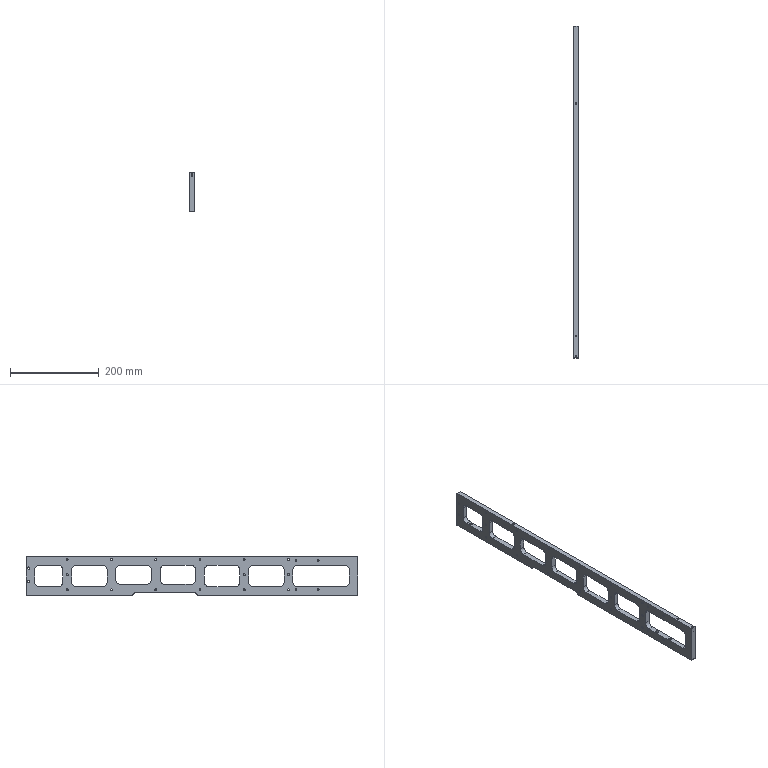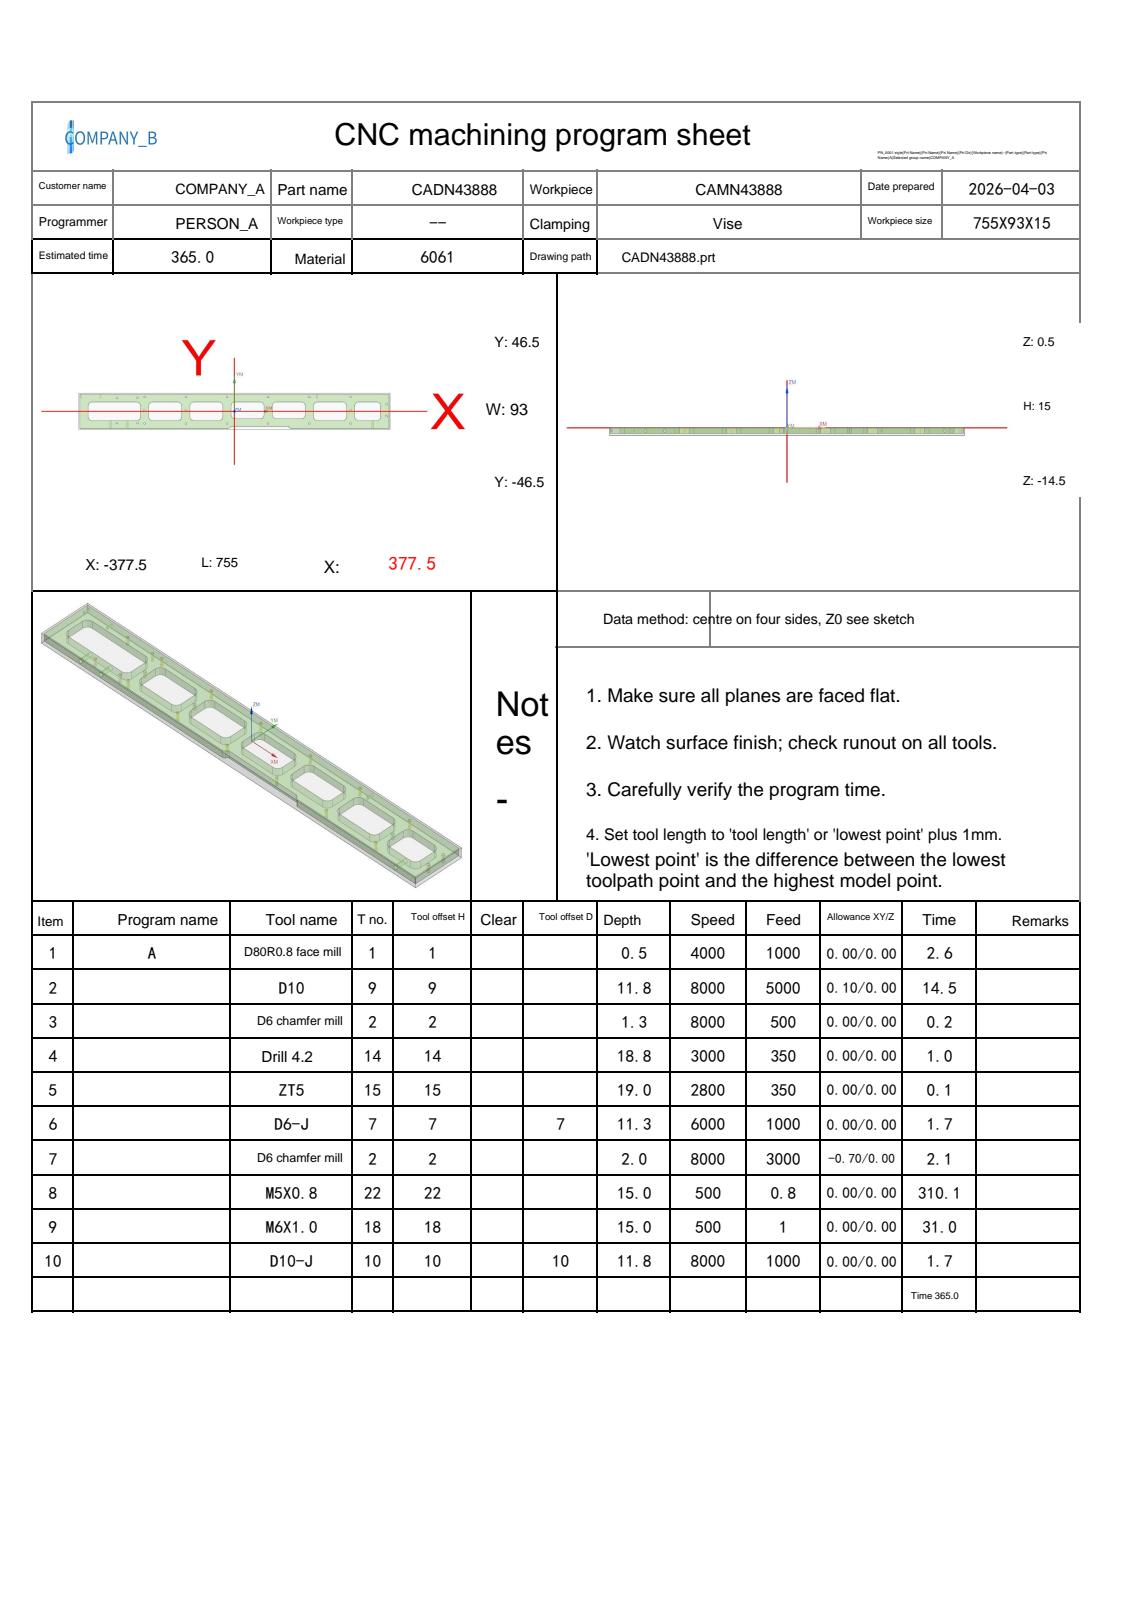NC program | NX | posted by the shop | part box 11 x 750 x 88 mm
Lines 1 to 1861 of 2351, first 1298 of 1859 lines:
%
O0001
(Machine time: 686.22 MIN)
(===Total Tool:9===)
(T1=D80R0.8 face mill D=80.  R=0.8  D-  H01 Z=-0.   )
(T9=D10     D=10.  R=0.   D-  H09 Z=-11.3 )
(T2=D6 chamfer mill   D=6.   R=0.   D-  H02 Z=-1.5  )
(T14=drill 4.2  D=4.2  DR_a=118 D-  H14 Z=-18.26)
(T15=ZT5    D=5.   DR_a=118 D-  H15 Z=-18.5 )
(T7=D6-J    D=6.   R=0.   D7  H07 Z=-10.8 )
(T22=M5X0.8 D=4.2  DR_a=180 D-  H22 Z=-14.5 )
(T18=M6X1.0 D=5.   DR_a=180 D-  H18 Z=-14.5 )
(T10=D10-J  D=10.  R=0.   D10 H10 Z=-11.3 )
G80 G90 G17 G49 G40
G91 G28 Z0
M01
N1 T01 M06
(D80R0.8 face mill  D=80. R=0.8 H=01 ce=0.00 di=0.00)
G00 G90 G54 X-420. Y42. M03 S4000
G43 H01 Z20.
M08
Z2.
G01 Z0.0 F1000.
X-415.
X415.
Y0.0
X-415.
Y-42.
X415.
X420.
Z2.
G00 Z20.
G91 G28 Z0.0
M05
M09
G91 G28 Z0.0
M01
N2 T09 M06
(D10  D=10. R=0. H=09 ce=0.10 di=0.00)
G00 G90 G54 X0.0 Y49.1 M03 S8000
G43 H09 Z20.
M08
Z.5
G01 X374. Z.328 F5000.
G02 X380.1 Y43. Z.324 I0.0 J-6.1
G01 Y-43. Z.284
G02 X374. Y-49.1 Z.28 I-6.1 J0.0
G01 X137.165 Z.171
G02 X127.935 Y-43.1 Z.165 I0.0 J10.1
G01 X-5.935 Z.104
G02 X-15.165 Y-49.1 Z.099 I-9.23 J4.1
G01 X-374. Z-.066
G02 X-380.1 Y-43. Z-.071 I0.0 J6.1
G01 Y43. Z-.11
G02 X-374. Y49.1 Z-.115 I6.1 J0.0
G01 X374. Z-.459
G02 X380.1 Y43. Z-.463 I0.0 J-6.1
G01 Y-43. Z-.503
G02 X374. Y-49.1 Z-.507 I-6.1 J0.0
G01 X137.165 Z-.616
G02 X127.935 Y-43.1 Z-.621 I0.0 J10.1
G01 X-5.935 Z-.683
G02 X-15.165 Y-49.1 Z-.688 I-9.23 J4.1
G01 X-374. Z-.853
G02 X-380.1 Y-43. Z-.857 I0.0 J6.1
G01 Y43. Z-.897
G02 X-374. Y49.1 Z-.901 I6.1 J0.0
G01 X374. Z-1.245
G02 X380.1 Y43. Z-1.25 I0.0 J-6.1
G01 Y-43. Z-1.289
G02 X374. Y-49.1 Z-1.294 I-6.1 J0.0
G01 X137.165 Z-1.402
G02 X127.935 Y-43.1 Z-1.408 I0.0 J10.1
G01 X-5.935 Z-1.469
G02 X-15.165 Y-49.1 Z-1.475 I-9.23 J4.1
G01 X-374. Z-1.64
G02 X-380.1 Y-43. Z-1.644 I0.0 J6.1
G01 Y43. Z-1.684
G02 X-374. Y49.1 Z-1.688 I6.1 J0.0
G01 X374. Z-2.032
G02 X380.1 Y43. Z-2.036 I0.0 J-6.1
G01 Y-43. Z-2.076
G02 X374. Y-49.1 Z-2.08 I-6.1 J0.0
G01 X137.165 Z-2.189
G02 X127.935 Y-43.1 Z-2.195 I0.0 J10.1
G01 X-5.935 Z-2.256
G02 X-15.165 Y-49.1 Z-2.261 I-9.23 J4.1
G01 X-374. Z-2.426
G02 X-380.1 Y-43. Z-2.431 I0.0 J6.1
G01 Y43. Z-2.47
G02 X-374. Y49.1 Z-2.475 I6.1 J0.0
G01 X374. Z-2.819
G02 X380.1 Y43. Z-2.823 I0.0 J-6.1
G01 Y-43. Z-2.863
G02 X374. Y-49.1 Z-2.867 I-6.1 J0.0
G01 X137.165 Z-2.976
G02 X127.935 Y-43.1 Z-2.981 I0.0 J10.1
G01 X-5.935 Z-3.043
G02 X-15.165 Y-49.1 Z-3.048 I-9.23 J4.1
G01 X-374. Z-3.213
G02 X-380.1 Y-43. Z-3.217 I0.0 J6.1
G01 Y43. Z-3.257
G02 X-374. Y49.1 Z-3.261 I6.1 J0.0
G01 X374. Z-3.605
G02 X380.1 Y43. Z-3.61 I0.0 J-6.1
G01 Y-43. Z-3.649
G02 X374. Y-49.1 Z-3.654 I-6.1 J0.0
G01 X137.165 Z-3.762
G02 X127.935 Y-43.1 Z-3.768 I0.0 J10.1
G01 X-5.935 Z-3.829
G02 X-15.165 Y-49.1 Z-3.835 I-9.23 J4.1
G01 X-374. Z-4.
G02 X-380.1 Y-43. Z-4.004 I0.0 J6.1
G01 Y43. Z-4.044
G02 X-374. Y49.1 Z-4.048 I6.1 J0.0
G01 X374. Z-4.392
G02 X380.1 Y43. Z-4.396 I0.0 J-6.1
G01 Y-43. Z-4.436
G02 X374. Y-49.1 Z-4.44 I-6.1 J0.0
G01 X137.165 Z-4.549
G02 X127.935 Y-43.1 Z-4.555 I0.0 J10.1
G01 X-5.935 Z-4.616
G02 X-15.165 Y-49.1 Z-4.621 I-9.23 J4.1
G01 X-374. Z-4.786
G02 X-380.1 Y-43. Z-4.791 I0.0 J6.1
G01 Y43. Z-4.83
G02 X-374. Y49.1 Z-4.835 I6.1 J0.0
G01 X374. Z-5.179
G02 X380.1 Y43. Z-5.183 I0.0 J-6.1
G01 Y-43. Z-5.223
G02 X374. Y-49.1 Z-5.227 I-6.1 J0.0
G01 X137.165 Z-5.336
G02 X127.935 Y-43.1 Z-5.341 I0.0 J10.1
G01 X-5.935 Z-5.403
G02 X-15.165 Y-49.1 Z-5.408 I-9.23 J4.1
G01 X-374. Z-5.573
G02 X-380.1 Y-43. Z-5.577 I0.0 J6.1
G01 Y43. Z-5.617
G02 X-374. Y49.1 Z-5.621 I6.1 J0.0
G01 X374. Z-5.965
G02 X380.1 Y43. Z-5.97 I0.0 J-6.1
G01 Y-43. Z-6.009
G02 X374. Y-49.1 Z-6.014 I-6.1 J0.0
G01 X137.165 Z-6.122
G02 X127.935 Y-43.1 Z-6.128 I0.0 J10.1
G01 X-5.935 Z-6.189
G02 X-15.165 Y-49.1 Z-6.195 I-9.23 J4.1
G01 X-374. Z-6.36
G02 X-380.1 Y-43. Z-6.364 I0.0 J6.1
G01 Y43. Z-6.404
G02 X-374. Y49.1 Z-6.408 I6.1 J0.0
G01 X374. Z-6.752
G02 X380.1 Y43. Z-6.756 I0.0 J-6.1
G01 Y-43. Z-6.796
G02 X374. Y-49.1 Z-6.8 I-6.1 J0.0
G01 X137.165 Z-6.909
G02 X127.935 Y-43.1 Z-6.915 I0.0 J10.1
G01 X-5.935 Z-6.976
G02 X-15.165 Y-49.1 Z-6.981 I-9.23 J4.1
G01 X-374. Z-7.146
G02 X-380.1 Y-43. Z-7.151 I0.0 J6.1
G01 Y43. Z-7.19
G02 X-374. Y49.1 Z-7.195 I6.1 J0.0
G01 X374. Z-7.539
G02 X380.1 Y43. Z-7.543 I0.0 J-6.1
G01 Y-43. Z-7.583
G02 X374. Y-49.1 Z-7.587 I-6.1 J0.0
G01 X137.165 Z-7.696
G02 X127.935 Y-43.1 Z-7.701 I0.0 J10.1
G01 X-5.935 Z-7.763
G02 X-15.165 Y-49.1 Z-7.768 I-9.23 J4.1
G01 X-374. Z-7.933
G02 X-380.1 Y-43. Z-7.937 I0.0 J6.1
G01 Y43. Z-7.977
G02 X-374. Y49.1 Z-7.981 I6.1 J0.0
G01 X374. Z-8.325
G02 X380.1 Y43. Z-8.33 I0.0 J-6.1
G01 Y-43. Z-8.369
G02 X374. Y-49.1 Z-8.374 I-6.1 J0.0
G01 X137.165 Z-8.482
G02 X127.935 Y-43.1 Z-8.488 I0.0 J10.1
G01 X-5.935 Z-8.549
G02 X-15.165 Y-49.1 Z-8.555 I-9.23 J4.1
G01 X-374. Z-8.72
G02 X-380.1 Y-43. Z-8.724 I0.0 J6.1
G01 Y43. Z-8.764
G02 X-374. Y49.1 Z-8.768 I6.1 J0.0
G01 X374. Z-9.112
G02 X380.1 Y43. Z-9.116 I0.0 J-6.1
G01 Y-43. Z-9.156
G02 X374. Y-49.1 Z-9.16 I-6.1 J0.0
G01 X137.165 Z-9.269
G02 X127.935 Y-43.1 Z-9.275 I0.0 J10.1
G01 X-5.935 Z-9.336
G02 X-15.165 Y-49.1 Z-9.341 I-9.23 J4.1
G01 X-374. Z-9.506
G02 X-380.1 Y-43. Z-9.511 I0.0 J6.1
G01 Y43. Z-9.55
G02 X-374. Y49.1 Z-9.555 I6.1 J0.0
G01 X374. Z-9.899
G02 X380.1 Y43. Z-9.903 I0.0 J-6.1
G01 Y-43. Z-9.943
G02 X374. Y-49.1 Z-9.947 I-6.1 J0.0
G01 X137.165 Z-10.056
G02 X127.935 Y-43.1 Z-10.061 I0.0 J10.1
G01 X-5.935 Z-10.123
G02 X-15.165 Y-49.1 Z-10.128 I-9.23 J4.1
G01 X-374. Z-10.293
G02 X-380.1 Y-43. Z-10.297 I0.0 J6.1
G01 Y43. Z-10.337
G02 X-374. Y49.1 Z-10.341 I6.1 J0.0
G01 X374. Z-10.685
G02 X380.1 Y43. Z-10.69 I0.0 J-6.1
G01 Y-43. Z-10.729
G02 X374. Y-49.1 Z-10.734 I-6.1 J0.0
G01 X137.165 Z-10.842
G02 X127.935 Y-43.1 Z-10.848 I0.0 J10.1
G01 X-5.935 Z-10.909
G02 X-15.165 Y-49.1 Z-10.915 I-9.23 J4.1
G01 X-374. Z-11.08
G02 X-380.1 Y-43. Z-11.084 I0.0 J6.1
G01 Y43. Z-11.124
G02 X-374. Y49.1 Z-11.128 I6.1 J0.0
G01 X0.0 Z-11.3
X374.
G02 X380.1 Y43. I0.0 J-6.1
G01 Y-43.
G02 X374. Y-49.1 I-6.1 J0.0
G01 X137.165
G02 X127.935 Y-43.1 I0.0 J10.1
G01 X-5.935
G02 X-15.165 Y-49.1 I-9.23 J4.1
G01 X-374.
G02 X-380.1 Y-43. I0.0 J6.1
G01 Y43.
G02 X-374. Y49.1 I6.1 J0.0
G01 X0.0
X.5
Z-10.3
G00 Z20.
G00 G90 X-291.5 Y-18.9 M03 S6000
Z20.
Z.5
G01 X-238. Z.413 F4000.
G03 X-233.1 Y-14. Z.4 I0.0 J4.9
G01 Y14. Z.354
G03 X-238. Y18.9 Z.342 I-4.9 J0.0
G01 X-345. Z.167
G03 X-349.9 Y14. Z.154 I0.0 J-4.9
G01 Y-14. Z.109
G03 X-345. Y-18.9 Z.096 I4.9 J0.0
G01 X-238. Z-.079
G03 X-233.1 Y-14. Z-.091 I0.0 J4.9
G01 Y14. Z-.137
G03 X-238. Y18.9 Z-.15 I-4.9 J0.0
G01 X-345. Z-.324
G03 X-349.9 Y14. Z-.337 I0.0 J-4.9
G01 Y-14. Z-.383
G03 X-345. Y-18.9 Z-.395 I4.9 J0.0
G01 X-238. Z-.57
G03 X-233.1 Y-14. Z-.583 I0.0 J4.9
G01 Y14. Z-.628
G03 X-238. Y18.9 Z-.641 I-4.9 J0.0
G01 X-345. Z-.816
G03 X-349.9 Y14. Z-.828 I0.0 J-4.9
G01 Y-14. Z-.874
G03 X-345. Y-18.9 Z-.887 I4.9 J0.0
G01 X-238. Z-1.061
G03 X-233.1 Y-14. Z-1.074 I0.0 J4.9
G01 Y14. Z-1.12
G03 X-238. Y18.9 Z-1.132 I-4.9 J0.0
G01 X-345. Z-1.307
G03 X-349.9 Y14. Z-1.32 I0.0 J-4.9
G01 Y-14. Z-1.365
G03 X-345. Y-18.9 Z-1.378 I4.9 J0.0
G01 X-238. Z-1.553
G03 X-233.1 Y-14. Z-1.565 I0.0 J4.9
G01 Y14. Z-1.611
G03 X-238. Y18.9 Z-1.623 I-4.9 J0.0
G01 X-345. Z-1.798
G03 X-349.9 Y14. Z-1.811 I0.0 J-4.9
G01 Y-14. Z-1.857
G03 X-345. Y-18.9 Z-1.869 I4.9 J0.0
G01 X-238. Z-2.044
G03 X-233.1 Y-14. Z-2.056 I0.0 J4.9
G01 Y14. Z-2.102
G03 X-238. Y18.9 Z-2.115 I-4.9 J0.0
G01 X-345. Z-2.29
G03 X-349.9 Y14. Z-2.302 I0.0 J-4.9
G01 Y-14. Z-2.348
G03 X-345. Y-18.9 Z-2.36 I4.9 J0.0
G01 X-238. Z-2.535
G03 X-233.1 Y-14. Z-2.548 I0.0 J4.9
G01 Y14. Z-2.594
G03 X-238. Y18.9 Z-2.606 I-4.9 J0.0
G01 X-345. Z-2.781
G03 X-349.9 Y14. Z-2.793 I0.0 J-4.9
G01 Y-14. Z-2.839
G03 X-345. Y-18.9 Z-2.852 I4.9 J0.0
G01 X-238. Z-3.027
G03 X-233.1 Y-14. Z-3.039 I0.0 J4.9
G01 Y14. Z-3.085
G03 X-238. Y18.9 Z-3.097 I-4.9 J0.0
G01 X-345. Z-3.272
G03 X-349.9 Y14. Z-3.285 I0.0 J-4.9
G01 Y-14. Z-3.33
G03 X-345. Y-18.9 Z-3.343 I4.9 J0.0
G01 X-238. Z-3.518
G03 X-233.1 Y-14. Z-3.53 I0.0 J4.9
G01 Y14. Z-3.576
G03 X-238. Y18.9 Z-3.589 I-4.9 J0.0
G01 X-345. Z-3.763
G03 X-349.9 Y14. Z-3.776 I0.0 J-4.9
G01 Y-14. Z-3.822
G03 X-345. Y-18.9 Z-3.834 I4.9 J0.0
G01 X-238. Z-4.009
G03 X-233.1 Y-14. Z-4.022 I0.0 J4.9
G01 Y14. Z-4.067
G03 X-238. Y18.9 Z-4.08 I-4.9 J0.0
G01 X-345. Z-4.255
G03 X-349.9 Y14. Z-4.267 I0.0 J-4.9
G01 Y-14. Z-4.313
G03 X-345. Y-18.9 Z-4.326 I4.9 J0.0
G01 X-238. Z-4.5
G03 X-233.1 Y-14. Z-4.513 I0.0 J4.9
G01 Y14. Z-4.559
G03 X-238. Y18.9 Z-4.571 I-4.9 J0.0
G01 X-345. Z-4.746
G03 X-349.9 Y14. Z-4.759 I0.0 J-4.9
G01 Y-14. Z-4.804
G03 X-345. Y-18.9 Z-4.817 I4.9 J0.0
G01 X-238. Z-4.992
G03 X-233.1 Y-14. Z-5.004 I0.0 J4.9
G01 Y14. Z-5.05
G03 X-238. Y18.9 Z-5.063 I-4.9 J0.0
G01 X-345. Z-5.237
G03 X-349.9 Y14. Z-5.25 I0.0 J-4.9
G01 Y-14. Z-5.296
G03 X-345. Y-18.9 Z-5.308 I4.9 J0.0
G01 X-238. Z-5.483
G03 X-233.1 Y-14. Z-5.496 I0.0 J4.9
G01 Y14. Z-5.541
G03 X-238. Y18.9 Z-5.554 I-4.9 J0.0
G01 X-345. Z-5.729
G03 X-349.9 Y14. Z-5.741 I0.0 J-4.9
G01 Y-14. Z-5.787
G03 X-345. Y-18.9 Z-5.8 I4.9 J0.0
G01 X-238. Z-5.974
G03 X-233.1 Y-14. Z-5.987 I0.0 J4.9
G01 Y14. Z-6.033
G03 X-238. Y18.9 Z-6.045 I-4.9 J0.0
G01 X-345. Z-6.22
G03 X-349.9 Y14. Z-6.233 I0.0 J-4.9
G01 Y-14. Z-6.278
G03 X-345. Y-18.9 Z-6.291 I4.9 J0.0
G01 X-238. Z-6.466
G03 X-233.1 Y-14. Z-6.478 I0.0 J4.9
G01 Y14. Z-6.524
G03 X-238. Y18.9 Z-6.537 I-4.9 J0.0
G01 X-345. Z-6.711
G03 X-349.9 Y14. Z-6.724 I0.0 J-4.9
G01 Y-14. Z-6.77
G03 X-345. Y-18.9 Z-6.782 I4.9 J0.0
G01 X-238. Z-6.957
G03 X-233.1 Y-14. Z-6.97 I0.0 J4.9
G01 Y14. Z-7.015
G03 X-238. Y18.9 Z-7.028 I-4.9 J0.0
G01 X-345. Z-7.203
G03 X-349.9 Y14. Z-7.215 I0.0 J-4.9
G01 Y-14. Z-7.261
G03 X-345. Y-18.9 Z-7.273 I4.9 J0.0
G01 X-238. Z-7.448
G03 X-233.1 Y-14. Z-7.461 I0.0 J4.9
G01 Y14. Z-7.507
G03 X-238. Y18.9 Z-7.519 I-4.9 J0.0
G01 X-345. Z-7.694
G03 X-349.9 Y14. Z-7.706 I0.0 J-4.9
G01 Y-14. Z-7.752
G03 X-345. Y-18.9 Z-7.765 I4.9 J0.0
G01 X-238. Z-7.94
G03 X-233.1 Y-14. Z-7.952 I0.0 J4.9
G01 Y14. Z-7.998
G03 X-238. Y18.9 Z-8.01 I-4.9 J0.0
G01 X-345. Z-8.185
G03 X-349.9 Y14. Z-8.198 I0.0 J-4.9
G01 Y-14. Z-8.244
G03 X-345. Y-18.9 Z-8.256 I4.9 J0.0
G01 X-238. Z-8.431
G03 X-233.1 Y-14. Z-8.443 I0.0 J4.9
G01 Y14. Z-8.489
G03 X-238. Y18.9 Z-8.502 I-4.9 J0.0
G01 X-345. Z-8.677
G03 X-349.9 Y14. Z-8.689 I0.0 J-4.9
G01 Y-14. Z-8.735
G03 X-345. Y-18.9 Z-8.747 I4.9 J0.0
G01 X-238. Z-8.922
G03 X-233.1 Y-14. Z-8.935 I0.0 J4.9
G01 Y14. Z-8.98
G03 X-238. Y18.9 Z-8.993 I-4.9 J0.0
G01 X-345. Z-9.168
G03 X-349.9 Y14. Z-9.18 I0.0 J-4.9
G01 Y-14. Z-9.226
G03 X-345. Y-18.9 Z-9.239 I4.9 J0.0
G01 X-238. Z-9.413
G03 X-233.1 Y-14. Z-9.426 I0.0 J4.9
G01 Y14. Z-9.472
G03 X-238. Y18.9 Z-9.484 I-4.9 J0.0
G01 X-345. Z-9.659
G03 X-349.9 Y14. Z-9.672 I0.0 J-4.9
G01 Y-14. Z-9.717
G03 X-345. Y-18.9 Z-9.73 I4.9 J0.0
G01 X-238. Z-9.905
G03 X-233.1 Y-14. Z-9.917 I0.0 J4.9
G01 Y14. Z-9.963
G03 X-238. Y18.9 Z-9.976 I-4.9 J0.0
G01 X-345. Z-10.15
G03 X-349.9 Y14. Z-10.163 I0.0 J-4.9
G01 Y-14. Z-10.209
G03 X-345. Y-18.9 Z-10.221 I4.9 J0.0
G01 X-238. Z-10.396
G03 X-233.1 Y-14. Z-10.409 I0.0 J4.9
G01 Y14. Z-10.454
G03 X-238. Y18.9 Z-10.467 I-4.9 J0.0
G01 X-345. Z-10.642
G03 X-349.9 Y14. Z-10.654 I0.0 J-4.9
G01 Y-14. Z-10.7
G03 X-345. Y-18.9 Z-10.713 I4.9 J0.0
G01 X-291.5 Z-10.8
X-238.
G03 X-233.1 Y-14. I0.0 J4.9
G01 Y14.
G03 X-238. Y18.9 I-4.9 J0.0
G01 X-345.
G03 X-349.9 Y14. I0.0 J-4.9
G01 Y-14.
G03 X-345. Y-18.9 I4.9 J0.0
G01 X-291.5
X-291.
Z-9.8
G00 Z20.
G00 G90 X-168. Y18.9 M03 S6000
Z20.
Z.5
G01 X-198. Z.429 F4000.
G03 X-202.9 Y14. Z.41 I0.0 J-4.9
G01 Y-14. Z.344
G03 X-198. Y-18.9 Z.326 I4.9 J0.0
G01 X-138. Z.183
G03 X-133.1 Y-14. Z.165 I0.0 J4.9
G01 Y14. Z.098
G03 X-138. Y18.9 Z.08 I-4.9 J0.0
G01 X-198. Z-.063
G03 X-202.9 Y14. Z-.081 I0.0 J-4.9
G01 Y-14. Z-.147
G03 X-198. Y-18.9 Z-.166 I4.9 J0.0
G01 X-138. Z-.308
G03 X-133.1 Y-14. Z-.327 I0.0 J4.9
G01 Y14. Z-.393
G03 X-138. Y18.9 Z-.411 I-4.9 J0.0
G01 X-198. Z-.554
G03 X-202.9 Y14. Z-.572 I0.0 J-4.9
G01 Y-14. Z-.639
G03 X-198. Y-18.9 Z-.657 I4.9 J0.0
G01 X-138. Z-.8
G03 X-133.1 Y-14. Z-.818 I0.0 J4.9
G01 Y14. Z-.884
G03 X-138. Y18.9 Z-.903 I-4.9 J0.0
G01 X-198. Z-1.045
G03 X-202.9 Y14. Z-1.063 I0.0 J-4.9
G01 Y-14. Z-1.13
G03 X-198. Y-18.9 Z-1.148 I4.9 J0.0
G01 X-138. Z-1.291
G03 X-133.1 Y-14. Z-1.309 I0.0 J4.9
G01 Y14. Z-1.376
G03 X-138. Y18.9 Z-1.394 I-4.9 J0.0
G01 X-198. Z-1.536
G03 X-202.9 Y14. Z-1.555 I0.0 J-4.9
G01 Y-14. Z-1.621
G03 X-198. Y-18.9 Z-1.64 I4.9 J0.0
G01 X-138. Z-1.782
G03 X-133.1 Y-14. Z-1.8 I0.0 J4.9
G01 Y14. Z-1.867
G03 X-138. Y18.9 Z-1.885 I-4.9 J0.0
G01 X-198. Z-2.028
G03 X-202.9 Y14. Z-2.046 I0.0 J-4.9
G01 Y-14. Z-2.113
G03 X-198. Y-18.9 Z-2.131 I4.9 J0.0
G01 X-138. Z-2.273
G03 X-133.1 Y-14. Z-2.292 I0.0 J4.9
G01 Y14. Z-2.358
G03 X-138. Y18.9 Z-2.377 I-4.9 J0.0
G01 X-198. Z-2.519
G03 X-202.9 Y14. Z-2.537 I0.0 J-4.9
G01 Y-14. Z-2.604
G03 X-198. Y-18.9 Z-2.622 I4.9 J0.0
G01 X-138. Z-2.765
G03 X-133.1 Y-14. Z-2.783 I0.0 J4.9
G01 Y14. Z-2.85
G03 X-138. Y18.9 Z-2.868 I-4.9 J0.0
G01 X-198. Z-3.01
G03 X-202.9 Y14. Z-3.029 I0.0 J-4.9
G01 Y-14. Z-3.095
G03 X-198. Y-18.9 Z-3.114 I4.9 J0.0
G01 X-138. Z-3.256
G03 X-133.1 Y-14. Z-3.274 I0.0 J4.9
G01 Y14. Z-3.341
G03 X-138. Y18.9 Z-3.359 I-4.9 J0.0
G01 X-198. Z-3.502
G03 X-202.9 Y14. Z-3.52 I0.0 J-4.9
G01 Y-14. Z-3.587
G03 X-198. Y-18.9 Z-3.605 I4.9 J0.0
G01 X-138. Z-3.747
G03 X-133.1 Y-14. Z-3.766 I0.0 J4.9
G01 Y14. Z-3.832
G03 X-138. Y18.9 Z-3.85 I-4.9 J0.0
G01 X-198. Z-3.993
G03 X-202.9 Y14. Z-4.011 I0.0 J-4.9
G01 Y-14. Z-4.078
G03 X-198. Y-18.9 Z-4.096 I4.9 J0.0
G01 X-138. Z-4.239
G03 X-133.1 Y-14. Z-4.257 I0.0 J4.9
G01 Y14. Z-4.323
G03 X-138. Y18.9 Z-4.342 I-4.9 J0.0
G01 X-198. Z-4.484
G03 X-202.9 Y14. Z-4.503 I0.0 J-4.9
G01 Y-14. Z-4.569
G03 X-198. Y-18.9 Z-4.587 I4.9 J0.0
G01 X-138. Z-4.73
G03 X-133.1 Y-14. Z-4.748 I0.0 J4.9
G01 Y14. Z-4.815
G03 X-138. Y18.9 Z-4.833 I-4.9 J0.0
G01 X-198. Z-4.976
G03 X-202.9 Y14. Z-4.994 I0.0 J-4.9
G01 Y-14. Z-5.06
G03 X-198. Y-18.9 Z-5.079 I4.9 J0.0
G01 X-138. Z-5.221
G03 X-133.1 Y-14. Z-5.24 I0.0 J4.9
G01 Y14. Z-5.306
G03 X-138. Y18.9 Z-5.324 I-4.9 J0.0
G01 X-198. Z-5.467
G03 X-202.9 Y14. Z-5.485 I0.0 J-4.9
G01 Y-14. Z-5.552
G03 X-198. Y-18.9 Z-5.57 I4.9 J0.0
G01 X-138. Z-5.713
G03 X-133.1 Y-14. Z-5.731 I0.0 J4.9
G01 Y14. Z-5.797
G03 X-138. Y18.9 Z-5.816 I-4.9 J0.0
G01 X-198. Z-5.958
G03 X-202.9 Y14. Z-5.977 I0.0 J-4.9
G01 Y-14. Z-6.043
G03 X-198. Y-18.9 Z-6.061 I4.9 J0.0
G01 X-138. Z-6.204
G03 X-133.1 Y-14. Z-6.222 I0.0 J4.9
G01 Y14. Z-6.289
G03 X-138. Y18.9 Z-6.307 I-4.9 J0.0
G01 X-198. Z-6.45
G03 X-202.9 Y14. Z-6.468 I0.0 J-4.9
G01 Y-14. Z-6.534
G03 X-198. Y-18.9 Z-6.553 I4.9 J0.0
G01 X-138. Z-6.695
G03 X-133.1 Y-14. Z-6.713 I0.0 J4.9
G01 Y14. Z-6.78
G03 X-138. Y18.9 Z-6.798 I-4.9 J0.0
G01 X-198. Z-6.941
G03 X-202.9 Y14. Z-6.959 I0.0 J-4.9
G01 Y-14. Z-7.026
G03 X-198. Y-18.9 Z-7.044 I4.9 J0.0
G01 X-138. Z-7.186
G03 X-133.1 Y-14. Z-7.205 I0.0 J4.9
G01 Y14. Z-7.271
G03 X-138. Y18.9 Z-7.29 I-4.9 J0.0
G01 X-198. Z-7.432
G03 X-202.9 Y14. Z-7.45 I0.0 J-4.9
G01 Y-14. Z-7.517
G03 X-198. Y-18.9 Z-7.535 I4.9 J0.0
G01 X-138. Z-7.678
G03 X-133.1 Y-14. Z-7.696 I0.0 J4.9
G01 Y14. Z-7.763
G03 X-138. Y18.9 Z-7.781 I-4.9 J0.0
G01 X-198. Z-7.923
G03 X-202.9 Y14. Z-7.942 I0.0 J-4.9
G01 Y-14. Z-8.008
G03 X-198. Y-18.9 Z-8.027 I4.9 J0.0
G01 X-138. Z-8.169
G03 X-133.1 Y-14. Z-8.187 I0.0 J4.9
G01 Y14. Z-8.254
G03 X-138. Y18.9 Z-8.272 I-4.9 J0.0
G01 X-198. Z-8.415
G03 X-202.9 Y14. Z-8.433 I0.0 J-4.9
G01 Y-14. Z-8.5
G03 X-198. Y-18.9 Z-8.518 I4.9 J0.0
G01 X-138. Z-8.66
G03 X-133.1 Y-14. Z-8.679 I0.0 J4.9
G01 Y14. Z-8.745
G03 X-138. Y18.9 Z-8.764 I-4.9 J0.0
G01 X-198. Z-8.906
G03 X-202.9 Y14. Z-8.924 I0.0 J-4.9
G01 Y-14. Z-8.991
G03 X-198. Y-18.9 Z-9.009 I4.9 J0.0
G01 X-138. Z-9.152
G03 X-133.1 Y-14. Z-9.17 I0.0 J4.9
G01 Y14. Z-9.237
G03 X-138. Y18.9 Z-9.255 I-4.9 J0.0
G01 X-198. Z-9.397
G03 X-202.9 Y14. Z-9.416 I0.0 J-4.9
G01 Y-14. Z-9.482
G03 X-198. Y-18.9 Z-9.5 I4.9 J0.0
G01 X-138. Z-9.643
G03 X-133.1 Y-14. Z-9.661 I0.0 J4.9
G01 Y14. Z-9.728
G03 X-138. Y18.9 Z-9.746 I-4.9 J0.0
G01 X-198. Z-9.889
G03 X-202.9 Y14. Z-9.907 I0.0 J-4.9
G01 Y-14. Z-9.973
G03 X-198. Y-18.9 Z-9.992 I4.9 J0.0
G01 X-138. Z-10.134
G03 X-133.1 Y-14. Z-10.153 I0.0 J4.9
G01 Y14. Z-10.219
G03 X-138. Y18.9 Z-10.237 I-4.9 J0.0
G01 X-198. Z-10.38
G03 X-202.9 Y14. Z-10.398 I0.0 J-4.9
G01 Y-14. Z-10.465
G03 X-198. Y-18.9 Z-10.483 I4.9 J0.0
G01 X-138. Z-10.626
G03 X-133.1 Y-14. Z-10.644 I0.0 J4.9
G01 Y14. Z-10.71
G03 X-138. Y18.9 Z-10.729 I-4.9 J0.0
G01 X-168. Z-10.8
X-198.
G03 X-202.9 Y14. I0.0 J-4.9
G01 Y-14.
G03 X-198. Y-18.9 I4.9 J0.0
G01 X-138.
G03 X-133.1 Y-14. I0.0 J4.9
G01 Y14.
G03 X-138. Y18.9 I-4.9 J0.0
G01 X-168.
X-168.5
Z-9.8
G00 Z20.
X-68.
Z.5
G01 X-98. Z.429
G03 X-102.9 Y14. Z.41 I0.0 J-4.9
G01 Y-14. Z.344
G03 X-98. Y-18.9 Z.326 I4.9 J0.0
G01 X-38. Z.183
G03 X-33.1 Y-14. Z.165 I0.0 J4.9
G01 Y14. Z.098
G03 X-38. Y18.9 Z.08 I-4.9 J0.0
G01 X-98. Z-.063
G03 X-102.9 Y14. Z-.081 I0.0 J-4.9
G01 Y-14. Z-.147
G03 X-98. Y-18.9 Z-.166 I4.9 J0.0
G01 X-38. Z-.308
G03 X-33.1 Y-14. Z-.327 I0.0 J4.9
G01 Y14. Z-.393
G03 X-38. Y18.9 Z-.411 I-4.9 J0.0
G01 X-98. Z-.554
G03 X-102.9 Y14. Z-.572 I0.0 J-4.9
G01 Y-14. Z-.639
G03 X-98. Y-18.9 Z-.657 I4.9 J0.0
G01 X-38. Z-.8
G03 X-33.1 Y-14. Z-.818 I0.0 J4.9
G01 Y14. Z-.884
G03 X-38. Y18.9 Z-.903 I-4.9 J0.0
G01 X-98. Z-1.045
G03 X-102.9 Y14. Z-1.063 I0.0 J-4.9
G01 Y-14. Z-1.13
G03 X-98. Y-18.9 Z-1.148 I4.9 J0.0
G01 X-38. Z-1.291
G03 X-33.1 Y-14. Z-1.309 I0.0 J4.9
G01 Y14. Z-1.376
G03 X-38. Y18.9 Z-1.394 I-4.9 J0.0
G01 X-98. Z-1.536
G03 X-102.9 Y14. Z-1.555 I0.0 J-4.9
G01 Y-14. Z-1.621
G03 X-98. Y-18.9 Z-1.64 I4.9 J0.0
G01 X-38. Z-1.782
G03 X-33.1 Y-14. Z-1.8 I0.0 J4.9
G01 Y14. Z-1.867
G03 X-38. Y18.9 Z-1.885 I-4.9 J0.0
G01 X-98. Z-2.028
G03 X-102.9 Y14. Z-2.046 I0.0 J-4.9
G01 Y-14. Z-2.113
G03 X-98. Y-18.9 Z-2.131 I4.9 J0.0
G01 X-38. Z-2.273
G03 X-33.1 Y-14. Z-2.292 I0.0 J4.9
G01 Y14. Z-2.358
G03 X-38. Y18.9 Z-2.377 I-4.9 J0.0
G01 X-98. Z-2.519
G03 X-102.9 Y14. Z-2.537 I0.0 J-4.9
G01 Y-14. Z-2.604
G03 X-98. Y-18.9 Z-2.622 I4.9 J0.0
G01 X-38. Z-2.765
G03 X-33.1 Y-14. Z-2.783 I0.0 J4.9
G01 Y14. Z-2.85
G03 X-38. Y18.9 Z-2.868 I-4.9 J0.0
G01 X-98. Z-3.01
G03 X-102.9 Y14. Z-3.029 I0.0 J-4.9
G01 Y-14. Z-3.095
G03 X-98. Y-18.9 Z-3.114 I4.9 J0.0
G01 X-38. Z-3.256
G03 X-33.1 Y-14. Z-3.274 I0.0 J4.9
G01 Y14. Z-3.341
G03 X-38. Y18.9 Z-3.359 I-4.9 J0.0
G01 X-98. Z-3.502
G03 X-102.9 Y14. Z-3.52 I0.0 J-4.9
G01 Y-14. Z-3.587
G03 X-98. Y-18.9 Z-3.605 I4.9 J0.0
G01 X-38. Z-3.747
G03 X-33.1 Y-14. Z-3.766 I0.0 J4.9
G01 Y14. Z-3.832
G03 X-38. Y18.9 Z-3.85 I-4.9 J0.0
G01 X-98. Z-3.993
G03 X-102.9 Y14. Z-4.011 I0.0 J-4.9
G01 Y-14. Z-4.078
G03 X-98. Y-18.9 Z-4.096 I4.9 J0.0
G01 X-38. Z-4.239
G03 X-33.1 Y-14. Z-4.257 I0.0 J4.9
G01 Y14. Z-4.323
G03 X-38. Y18.9 Z-4.342 I-4.9 J0.0
G01 X-98. Z-4.484
G03 X-102.9 Y14. Z-4.503 I0.0 J-4.9
G01 Y-14. Z-4.569
G03 X-98. Y-18.9 Z-4.587 I4.9 J0.0
G01 X-38. Z-4.73
G03 X-33.1 Y-14. Z-4.748 I0.0 J4.9
G01 Y14. Z-4.815
G03 X-38. Y18.9 Z-4.833 I-4.9 J0.0
G01 X-98. Z-4.976
G03 X-102.9 Y14. Z-4.994 I0.0 J-4.9
G01 Y-14. Z-5.06
G03 X-98. Y-18.9 Z-5.079 I4.9 J0.0
G01 X-38. Z-5.221
G03 X-33.1 Y-14. Z-5.24 I0.0 J4.9
G01 Y14. Z-5.306
G03 X-38. Y18.9 Z-5.324 I-4.9 J0.0
G01 X-98. Z-5.467
G03 X-102.9 Y14. Z-5.485 I0.0 J-4.9
G01 Y-14. Z-5.552
G03 X-98. Y-18.9 Z-5.57 I4.9 J0.0
G01 X-38. Z-5.713
G03 X-33.1 Y-14. Z-5.731 I0.0 J4.9
G01 Y14. Z-5.797
G03 X-38. Y18.9 Z-5.816 I-4.9 J0.0
G01 X-98. Z-5.958
G03 X-102.9 Y14. Z-5.977 I0.0 J-4.9
G01 Y-14. Z-6.043
G03 X-98. Y-18.9 Z-6.061 I4.9 J0.0
G01 X-38. Z-6.204
G03 X-33.1 Y-14. Z-6.222 I0.0 J4.9
G01 Y14. Z-6.289
G03 X-38. Y18.9 Z-6.307 I-4.9 J0.0
G01 X-98. Z-6.45
G03 X-102.9 Y14. Z-6.468 I0.0 J-4.9
G01 Y-14. Z-6.534
G03 X-98. Y-18.9 Z-6.553 I4.9 J0.0
G01 X-38. Z-6.695
G03 X-33.1 Y-14. Z-6.713 I0.0 J4.9
G01 Y14. Z-6.78
G03 X-38. Y18.9 Z-6.798 I-4.9 J0.0
G01 X-98. Z-6.941
G03 X-102.9 Y14. Z-6.959 I0.0 J-4.9
G01 Y-14. Z-7.026
G03 X-98. Y-18.9 Z-7.044 I4.9 J0.0
G01 X-38. Z-7.186
G03 X-33.1 Y-14. Z-7.205 I0.0 J4.9
G01 Y14. Z-7.271
G03 X-38. Y18.9 Z-7.29 I-4.9 J0.0
G01 X-98. Z-7.432
G03 X-102.9 Y14. Z-7.45 I0.0 J-4.9
G01 Y-14. Z-7.517
G03 X-98. Y-18.9 Z-7.535 I4.9 J0.0
G01 X-38. Z-7.678
G03 X-33.1 Y-14. Z-7.696 I0.0 J4.9
G01 Y14. Z-7.763
G03 X-38. Y18.9 Z-7.781 I-4.9 J0.0
G01 X-98. Z-7.923
G03 X-102.9 Y14. Z-7.942 I0.0 J-4.9
G01 Y-14. Z-8.008
G03 X-98. Y-18.9 Z-8.027 I4.9 J0.0
G01 X-38. Z-8.169
G03 X-33.1 Y-14. Z-8.187 I0.0 J4.9
G01 Y14. Z-8.254
G03 X-38. Y18.9 Z-8.272 I-4.9 J0.0
G01 X-98. Z-8.415
G03 X-102.9 Y14. Z-8.433 I0.0 J-4.9
G01 Y-14. Z-8.5
G03 X-98. Y-18.9 Z-8.518 I4.9 J0.0
G01 X-38. Z-8.66
G03 X-33.1 Y-14. Z-8.679 I0.0 J4.9
G01 Y14. Z-8.745
G03 X-38. Y18.9 Z-8.764 I-4.9 J0.0
G01 X-98. Z-8.906
G03 X-102.9 Y14. Z-8.924 I0.0 J-4.9
G01 Y-14. Z-8.991
G03 X-98. Y-18.9 Z-9.009 I4.9 J0.0
G01 X-38. Z-9.152
G03 X-33.1 Y-14. Z-9.17 I0.0 J4.9
G01 Y14. Z-9.237
G03 X-38. Y18.9 Z-9.255 I-4.9 J0.0
G01 X-98. Z-9.397
G03 X-102.9 Y14. Z-9.416 I0.0 J-4.9
G01 Y-14. Z-9.482
G03 X-98. Y-18.9 Z-9.5 I4.9 J0.0
G01 X-38. Z-9.643
G03 X-33.1 Y-14. Z-9.661 I0.0 J4.9
G01 Y14. Z-9.728
G03 X-38. Y18.9 Z-9.746 I-4.9 J0.0
G01 X-98. Z-9.889
G03 X-102.9 Y14. Z-9.907 I0.0 J-4.9
G01 Y-14. Z-9.973
G03 X-98. Y-18.9 Z-9.992 I4.9 J0.0
G01 X-38. Z-10.134
G03 X-33.1 Y-14. Z-10.153 I0.0 J4.9
G01 Y14. Z-10.219
G03 X-38. Y18.9 Z-10.237 I-4.9 J0.0
G01 X-98. Z-10.38
G03 X-102.9 Y14. Z-10.398 I0.0 J-4.9
G01 Y-14. Z-10.465
G03 X-98. Y-18.9 Z-10.483 I4.9 J0.0
G01 X-38. Z-10.626
G03 X-33.1 Y-14. Z-10.644 I0.0 J4.9
G01 Y14. Z-10.71
G03 X-38. Y18.9 Z-10.729 I-4.9 J0.0
G01 X-68. Z-10.8
X-98.
G03 X-102.9 Y14. I0.0 J-4.9
G01 Y-14.
G03 X-98. Y-18.9 I4.9 J0.0
G01 X-38.
G03 X-33.1 Y-14. I0.0 J4.9
G01 Y14.
G03 X-38. Y18.9 I-4.9 J0.0
G01 X-68.
X-68.5
Z-9.8
G00 Z20.
X232. Y-18.9
Z.5
G01 X262. Z.429
G03 X266.9 Y-14. Z.41 I0.0 J4.9
G01 Y14. Z.344
G03 X262. Y18.9 Z.326 I-4.9 J0.0
G01 X202. Z.183
G03 X197.1 Y14. Z.165 I0.0 J-4.9
G01 Y-14. Z.098
G03 X202. Y-18.9 Z.08 I4.9 J0.0
G01 X262. Z-.063
G03 X266.9 Y-14. Z-.081 I0.0 J4.9
G01 Y14. Z-.147
G03 X262. Y18.9 Z-.166 I-4.9 J0.0
G01 X202. Z-.308
G03 X197.1 Y14. Z-.327 I0.0 J-4.9
G01 Y-14. Z-.393
G03 X202. Y-18.9 Z-.411 I4.9 J0.0
G01 X262. Z-.554
G03 X266.9 Y-14. Z-.572 I0.0 J4.9
G01 Y14. Z-.639
G03 X262. Y18.9 Z-.657 I-4.9 J0.0
G01 X202. Z-.8
G03 X197.1 Y14. Z-.818 I0.0 J-4.9
G01 Y-14. Z-.884
G03 X202. Y-18.9 Z-.903 I4.9 J0.0
G01 X262. Z-1.045
G03 X266.9 Y-14. Z-1.063 I0.0 J4.9
G01 Y14. Z-1.13
G03 X262. Y18.9 Z-1.148 I-4.9 J0.0
G01 X202. Z-1.291
G03 X197.1 Y14. Z-1.309 I0.0 J-4.9
G01 Y-14. Z-1.376
G03 X202. Y-18.9 Z-1.394 I4.9 J0.0
G01 X262. Z-1.536
G03 X266.9 Y-14. Z-1.555 I0.0 J4.9
G01 Y14. Z-1.621
G03 X262. Y18.9 Z-1.64 I-4.9 J0.0
G01 X202. Z-1.782
G03 X197.1 Y14. Z-1.8 I0.0 J-4.9
G01 Y-14. Z-1.867
G03 X202. Y-18.9 Z-1.885 I4.9 J0.0
G01 X262. Z-2.028
G03 X266.9 Y-14. Z-2.046 I0.0 J4.9
G01 Y14. Z-2.113
G03 X262. Y18.9 Z-2.131 I-4.9 J0.0
G01 X202. Z-2.273
G03 X197.1 Y14. Z-2.292 I0.0 J-4.9
G01 Y-14. Z-2.358
G03 X202. Y-18.9 Z-2.377 I4.9 J0.0
G01 X262. Z-2.519
G03 X266.9 Y-14. Z-2.537 I0.0 J4.9
G01 Y14. Z-2.604
G03 X262. Y18.9 Z-2.622 I-4.9 J0.0
G01 X202. Z-2.765
G03 X197.1 Y14. Z-2.783 I0.0 J-4.9
G01 Y-14. Z-2.85
G03 X202. Y-18.9 Z-2.868 I4.9 J0.0
G01 X262. Z-3.01
G03 X266.9 Y-14. Z-3.029 I0.0 J4.9
G01 Y14. Z-3.095
G03 X262. Y18.9 Z-3.114 I-4.9 J0.0
G01 X202. Z-3.256
G03 X197.1 Y14. Z-3.274 I0.0 J-4.9
G01 Y-14. Z-3.341
G03 X202. Y-18.9 Z-3.359 I4.9 J0.0
G01 X262. Z-3.502
G03 X266.9 Y-14. Z-3.52 I0.0 J4.9
G01 Y14. Z-3.587
G03 X262. Y18.9 Z-3.605 I-4.9 J0.0
G01 X202. Z-3.747
G03 X197.1 Y14. Z-3.766 I0.0 J-4.9
G01 Y-14. Z-3.832
G03 X202. Y-18.9 Z-3.85 I4.9 J0.0
G01 X262. Z-3.993
G03 X266.9 Y-14. Z-4.011 I0.0 J4.9
G01 Y14. Z-4.078
G03 X262. Y18.9 Z-4.096 I-4.9 J0.0
G01 X202. Z-4.239
G03 X197.1 Y14. Z-4.257 I0.0 J-4.9
G01 Y-14. Z-4.323
G03 X202. Y-18.9 Z-4.342 I4.9 J0.0
G01 X262. Z-4.484
G03 X266.9 Y-14. Z-4.503 I0.0 J4.9
G01 Y14. Z-4.569
G03 X262. Y18.9 Z-4.587 I-4.9 J0.0
G01 X202. Z-4.73
G03 X197.1 Y14. Z-4.748 I0.0 J-4.9
G01 Y-14. Z-4.815
G03 X202. Y-18.9 Z-4.833 I4.9 J0.0
G01 X262. Z-4.976
G03 X266.9 Y-14. Z-4.994 I0.0 J4.9
G01 Y14. Z-5.06
G03 X262. Y18.9 Z-5.079 I-4.9 J0.0
G01 X202. Z-5.221
G03 X197.1 Y14. Z-5.24 I0.0 J-4.9
G01 Y-14. Z-5.306
G03 X202. Y-18.9 Z-5.324 I4.9 J0.0
G01 X262. Z-5.467
G03 X266.9 Y-14. Z-5.485 I0.0 J4.9
G01 Y14. Z-5.552
G03 X262. Y18.9 Z-5.57 I-4.9 J0.0
G01 X202. Z-5.713
G03 X197.1 Y14. Z-5.731 I0.0 J-4.9
G01 Y-14. Z-5.797
G03 X202. Y-18.9 Z-5.816 I4.9 J0.0
G01 X262. Z-5.958
G03 X266.9 Y-14. Z-5.977 I0.0 J4.9
G01 Y14. Z-6.043
G03 X262. Y18.9 Z-6.061 I-4.9 J0.0
G01 X202. Z-6.204
G03 X197.1 Y14. Z-6.222 I0.0 J-4.9
G01 Y-14. Z-6.289
G03 X202. Y-18.9 Z-6.307 I4.9 J0.0
G01 X262. Z-6.45
G03 X266.9 Y-14. Z-6.468 I0.0 J4.9
G01 Y14. Z-6.534
G03 X262. Y18.9 Z-6.553 I-4.9 J0.0
G01 X202. Z-6.695
G03 X197.1 Y14. Z-6.713 I0.0 J-4.9
G01 Y-14. Z-6.78
G03 X202. Y-18.9 Z-6.798 I4.9 J0.0
G01 X262. Z-6.941
G03 X266.9 Y-14. Z-6.959 I0.0 J4.9
G01 Y14. Z-7.026
G03 X262. Y18.9 Z-7.044 I-4.9 J0.0
G01 X202. Z-7.186
G03 X197.1 Y14. Z-7.205 I0.0 J-4.9
G01 Y-14. Z-7.271
G03 X202. Y-18.9 Z-7.29 I4.9 J0.0
G01 X262. Z-7.432
G03 X266.9 Y-14. Z-7.45 I0.0 J4.9
G01 Y14. Z-7.517
G03 X262. Y18.9 Z-7.535 I-4.9 J0.0
G01 X202. Z-7.678
G03 X197.1 Y14. Z-7.696 I0.0 J-4.9
G01 Y-14. Z-7.763
G03 X202. Y-18.9 Z-7.781 I4.9 J0.0
G01 X262. Z-7.923
G03 X266.9 Y-14. Z-7.942 I0.0 J4.9
G01 Y14. Z-8.008
G03 X262. Y18.9 Z-8.027 I-4.9 J0.0
G01 X202. Z-8.169
G03 X197.1 Y14. Z-8.187 I0.0 J-4.9
G01 Y-14. Z-8.254
G03 X202. Y-18.9 Z-8.272 I4.9 J0.0
G01 X262. Z-8.415
G03 X266.9 Y-14. Z-8.433 I0.0 J4.9
G01 Y14. Z-8.5
G03 X262. Y18.9 Z-8.518 I-4.9 J0.0
G01 X202. Z-8.66
G03 X197.1 Y14. Z-8.679 I0.0 J-4.9
G01 Y-14. Z-8.745
G03 X202. Y-18.9 Z-8.764 I4.9 J0.0
G01 X262. Z-8.906
G03 X266.9 Y-14. Z-8.924 I0.0 J4.9
G01 Y14. Z-8.991
G03 X262. Y18.9 Z-9.009 I-4.9 J0.0
G01 X202. Z-9.152
G03 X197.1 Y14. Z-9.17 I0.0 J-4.9
G01 Y-14. Z-9.237
G03 X202. Y-18.9 Z-9.255 I4.9 J0.0
G01 X262. Z-9.397
G03 X266.9 Y-14. Z-9.416 I0.0 J4.9
G01 Y14. Z-9.482
G03 X262. Y18.9 Z-9.5 I-4.9 J0.0
G01 X202. Z-9.643
G03 X197.1 Y14. Z-9.661 I0.0 J-4.9
G01 Y-14. Z-9.728
G03 X202. Y-18.9 Z-9.746 I4.9 J0.0
G01 X262. Z-9.889
G03 X266.9 Y-14. Z-9.907 I0.0 J4.9
G01 Y14. Z-9.973
G03 X262. Y18.9 Z-9.992 I-4.9 J0.0
G01 X202. Z-10.134
G03 X197.1 Y14. Z-10.153 I0.0 J-4.9
G01 Y-14. Z-10.219
G03 X202. Y-18.9 Z-10.237 I4.9 J0.0
G01 X262. Z-10.38
G03 X266.9 Y-14. Z-10.398 I0.0 J4.9
G01 Y14. Z-10.465
G03 X262. Y18.9 Z-10.483 I-4.9 J0.0
G01 X202. Z-10.626
G03 X197.1 Y14. Z-10.644 I0.0 J-4.9
G01 Y-14. Z-10.71
G03 X202. Y-18.9 Z-10.729 I4.9 J0.0
G01 X232. Z-10.8
X262.
G03 X266.9 Y-14. I0.0 J4.9
G01 Y14.
G03 X262. Y18.9 I-4.9 J0.0
G01 X202.
G03 X197.1 Y14. I0.0 J-4.9
G01 Y-14.
G03 X202. Y-18.9 I4.9 J0.0
G01 X232.
X232.5
Z-9.8
G00 Z20.
G00 G90 X132. Y18.9 M03 S6000
Z20.
Z.5
G01 X102. Z.425 F4000.
G03 X97.1 Y14. Z.406 I0.0 J-4.9
G01 Y-9. Z.348
G03 X102. Y-13.9 Z.329 I4.9 J0.0
G01 X162. Z.179
G03 X166.9 Y-9. Z.16 I0.0 J4.9
G01 Y14. Z.103
G03 X162. Y18.9 Z.084 I-4.9 J0.0
G01 X102. Z-.066
G03 X97.1 Y14. Z-.085 I0.0 J-4.9
G01 Y-9. Z-.143
G03 X102. Y-13.9 Z-.162 I4.9 J0.0
G01 X162. Z-.312
G03 X166.9 Y-9. Z-.331 I0.0 J4.9
G01 Y14. Z-.388
G03 X162. Y18.9 Z-.408 I-4.9 J0.0
G01 X102. Z-.558
G03 X97.1 Y14. Z-.577 I0.0 J-4.9
G01 Y-9. Z-.634
G03 X102. Y-13.9 Z-.653 I4.9 J0.0
G01 X162. Z-.803
G03 X166.9 Y-9. Z-.822 I0.0 J4.9
G01 Y14. Z-.88
G03 X162. Y18.9 Z-.899 I-4.9 J0.0
G01 X102. Z-1.049
G03 X97.1 Y14. Z-1.068 I0.0 J-4.9
G01 Y-9. Z-1.125
G03 X102. Y-13.9 Z-1.145 I4.9 J0.0
G01 X162. Z-1.294
G03 X166.9 Y-9. Z-1.314 I0.0 J4.9
G01 Y14. Z-1.371
G03 X162. Y18.9 Z-1.39 I-4.9 J0.0
G01 X102. Z-1.54
G03 X97.1 Y14. Z-1.559 I0.0 J-4.9
G01 Y-9. Z-1.617
G03 X102. Y-13.9 Z-1.636 I4.9 J0.0
G01 X162. Z-1.786
G03 X166.9 Y-9. Z-1.805 I0.0 J4.9
G01 Y14. Z-1.862
G03 X162. Y18.9 Z-1.882 I-4.9 J0.0
G01 X102. Z-2.031
G03 X97.1 Y14. Z-2.051 I0.0 J-4.9
G01 Y-9. Z-2.108
G03 X102. Y-13.9 Z-2.127 I4.9 J0.0
G01 X162. Z-2.277
G03 X166.9 Y-9. Z-2.296 I0.0 J4.9
G01 Y14. Z-2.354
G03 X162. Y18.9 Z-2.373 I-4.9 J0.0
G01 X102. Z-2.523
G03 X97.1 Y14. Z-2.542 I0.0 J-4.9
G01 Y-9. Z-2.599
G03 X102. Y-13.9 Z-2.619 I4.9 J0.0
G01 X162. Z-2.768
G03 X166.9 Y-9. Z-2.788 I0.0 J4.9
G01 Y14. Z-2.845
G03 X162. Y18.9 Z-2.864 I-4.9 J0.0
G01 X102. Z-3.014
G03 X97.1 Y14. Z-3.033 I0.0 J-4.9
G01 Y-9. Z-3.091
G03 X102. Y-13.9 Z-3.11 I4.9 J0.0
G01 X162. Z-3.26
G03 X166.9 Y-9. Z-3.279 I0.0 J4.9
G01 Y14. Z-3.336
G03 X162. Y18.9 Z-3.356 I-4.9 J0.0
G01 X102. Z-3.505
G03 X97.1 Y14. Z-3.525 I0.0 J-4.9
G01 Y-9. Z-3.582
G03 X102. Y-13.9 Z-3.601 I4.9 J0.0
G01 X162. Z-3.751
G03 X166.9 Y-9. Z-3.77 I0.0 J4.9
G01 Y14. Z-3.828
G03 X162. Y18.9 Z-3.847 I-4.9 J0.0
G01 X102. Z-3.997
G03 X97.1 Y14. Z-4.016 I0.0 J-4.9
G01 Y-9. Z-4.073
G03 X102. Y-13.9 Z-4.092 I4.9 J0.0
G01 X162. Z-4.242
G03 X166.9 Y-9. Z-4.262 I0.0 J4.9
G01 Y14. Z-4.319
G03 X162. Y18.9 Z-4.338 I-4.9 J0.0
G01 X102. Z-4.488
G03 X97.1 Y14. Z-4.507 I0.0 J-4.9
G01 Y-9. Z-4.565
G03 X102. Y-13.9 Z-4.584 I4.9 J0.0
G01 X162. Z-4.734
G03 X166.9 Y-9. Z-4.753 I0.0 J4.9
G01 Y14. Z-4.81
G03 X162. Y18.9 Z-4.829 I-4.9 J0.0
G01 X102. Z-4.979
G03 X97.1 Y14. Z-4.998 I0.0 J-4.9
G01 Y-9. Z-5.056
G03 X102. Y-13.9 Z-5.075 I4.9 J0.0
G01 X162. Z-5.225
G03 X166.9 Y-9. Z-5.244 I0.0 J4.9
G01 Y14. Z-5.302
G03 X162. Y18.9 Z-5.321 I-4.9 J0.0
G01 X102. Z-5.471
G03 X97.1 Y14. Z-5.49 I0.0 J-4.9
G01 Y-9. Z-5.547
G03 X102. Y-13.9 Z-5.566 I4.9 J0.0
G01 X162. Z-5.716
G03 X166.9 Y-9. Z-5.735 I0.0 J4.9
G01 Y14. Z-5.793
G03 X162. Y18.9 Z-5.812 I-4.9 J0.0
G01 X102. Z-5.962
G03 X97.1 Y14. Z-5.981 I0.0 J-4.9
G01 Y-9. Z-6.038
G03 X102. Y-13.9 Z-6.058 I4.9 J0.0
G01 X162. Z-6.208
G03 X166.9 Y-9. Z-6.227 I0.0 J4.9
G01 Y14. Z-6.284
G03 X162. Y18.9 Z-6.303 I-4.9 J0.0
G01 X102. Z-6.453
G03 X97.1 Y14. Z-6.472 I0.0 J-4.9
G01 Y-9. Z-6.53
G03 X102. Y-13.9 Z-6.549 I4.9 J0.0
G01 X162. Z-6.699
G03 X166.9 Y-9. Z-6.718 I0.0 J4.9
G01 Y14. Z-6.775
G03 X162. Y18.9 Z-6.795 I-4.9 J0.0
G01 X102. Z-6.944
G03 X97.1 Y14. Z-6.964 I0.0 J-4.9
G01 Y-9. Z-7.021
G03 X102. Y-13.9 Z-7.04 I4.9 J0.0
G01 X162. Z-7.19
G03 X166.9 Y-9. Z-7.209 I0.0 J4.9
G01 Y14. Z-7.267
G03 X162. Y18.9 Z-7.286 I-4.9 J0.0
G01 X102. Z-7.436
G03 X97.1 Y14. Z-7.455 I0.0 J-4.9
G01 Y-9. Z-7.512
G03 X102. Y-13.9 Z-7.532 I4.9 J0.0
G01 X162. Z-7.681
G03 X166.9 Y-9. Z-7.701 I0.0 J4.9
G01 Y14. Z-7.758
G03 X162. Y18.9 Z-7.777 I-4.9 J0.0
G01 X102. Z-7.927
G03 X97.1 Y14. Z-7.946 I0.0 J-4.9
G01 Y-9. Z-8.004
G03 X102. Y-13.9 Z-8.023 I4.9 J0.0
G01 X162. Z-8.173
G03 X166.9 Y-9. Z-8.192 I0.0 J4.9
G01 Y14. Z-8.249
G03 X162. Y18.9 Z-8.269 I-4.9 J0.0
G01 X102. Z-8.418
G03 X97.1 Y14. Z-8.438 I0.0 J-4.9
G01 Y-9. Z-8.495
G03 X102. Y-13.9 Z-8.514 I4.9 J0.0
G01 X162. Z-8.664
G03 X166.9 Y-9. Z-8.683 I0.0 J4.9
G01 Y14. Z-8.741
G03 X162. Y18.9 Z-8.76 I-4.9 J0.0
G01 X102. Z-8.91
G03 X97.1 Y14. Z-8.929 I0.0 J-4.9
G01 Y-9. Z-8.986
G03 X102. Y-13.9 Z-9.006 I4.9 J0.0
G01 X162. Z-9.155
G03 X166.9 Y-9. Z-9.175 I0.0 J4.9
G01 Y14. Z-9.232
G03 X162. Y18.9 Z-9.251 I-4.9 J0.0
G01 X102. Z-9.401
G03 X97.1 Y14. Z-9.42 I0.0 J-4.9
G01 Y-9. Z-9.478
G03 X102. Y-13.9 Z-9.497 I4.9 J0.0
G01 X162. Z-9.647
G03 X166.9 Y-9. Z-9.666 I0.0 J4.9
G01 Y14. Z-9.723
G03 X162. Y18.9 Z-9.742 I-4.9 J0.0
G01 X102. Z-9.892
G03 X97.1 Y14. Z-9.912 I0.0 J-4.9
G01 Y-9. Z-9.969
G03 X102. Y-13.9 Z-9.988 I4.9 J0.0
G01 X162. Z-10.138
G03 X166.9 Y-9. Z-10.157 I0.0 J4.9
G01 Y14. Z-10.215
G03 X162. Y18.9 Z-10.234 I-4.9 J0.0
G01 X102. Z-10.384
G03 X97.1 Y14. Z-10.403 I0.0 J-4.9
G01 Y-9. Z-10.46
G03 X102. Y-13.9 Z-10.479 I4.9 J0.0
G01 X162. Z-10.629
G03 X166.9 Y-9. Z-10.648 I0.0 J4.9
G01 Y14. Z-10.706
G03 X162. Y18.9 Z-10.725 I-4.9 J0.0
G01 X132. Z-10.8
X102.
G03 X97.1 Y14. I0.0 J-4.9
G01 Y-9.
G03 X102. Y-13.9 I4.9 J0.0
G01 X162.
G03 X166.9 Y-9. I0.0 J4.9
G01 Y14.
G03 X162. Y18.9 I-4.9 J0.0
G01 X132.
X131.5
Z-9.8
G00 Z20.
X32.
Z.5
G01 X2. Z.425
G03 X-2.9 Y14. Z.406 I0.0 J-4.9
G01 Y-9. Z.348
G03 X2. Y-13.9 Z.329 I4.9 J0.0
G01 X62. Z.179
G03 X66.9 Y-9. Z.16 I0.0 J4.9
G01 Y14. Z.103
G03 X62. Y18.9 Z.084 I-4.9 J0.0
G01 X2. Z-.066
G03 X-2.9 Y14. Z-.085 I0.0 J-4.9
G01 Y-9. Z-.143
G03 X2. Y-13.9 Z-.162 I4.9 J0.0
G01 X62. Z-.312
G03 X66.9 Y-9. Z-.331 I0.0 J4.9
G01 Y14. Z-.388
G03 X62. Y18.9 Z-.408 I-4.9 J0.0
G01 X2. Z-.558
G03 X-2.9 Y14. Z-.577 I0.0 J-4.9
G01 Y-9. Z-.634
G03 X2. Y-13.9 Z-.653 I4.9 J0.0
G01 X62. Z-.803
G03 X66.9 Y-9. Z-.822 I0.0 J4.9
G01 Y14. Z-.88
G03 X62. Y18.9 Z-.899 I-4.9 J0.0
G01 X2. Z-1.049
G03 X-2.9 Y14. Z-1.068 I0.0 J-4.9
G01 Y-9. Z-1.125
G03 X2. Y-13.9 Z-1.145 I4.9 J0.0
G01 X62. Z-1.294
G03 X66.9 Y-9. Z-1.314 I0.0 J4.9
G01 Y14. Z-1.371
G03 X62. Y18.9 Z-1.39 I-4.9 J0.0
G01 X2. Z-1.54
G03 X-2.9 Y14. Z-1.559 I0.0 J-4.9
G01 Y-9. Z-1.617
G03 X2. Y-13.9 Z-1.636 I4.9 J0.0
G01 X62. Z-1.786
G03 X66.9 Y-9. Z-1.805 I0.0 J4.9
G01 Y14. Z-1.862
G03 X62. Y18.9 Z-1.882 I-4.9 J0.0
G01 X2. Z-2.031
G03 X-2.9 Y14. Z-2.051 I0.0 J-4.9
G01 Y-9. Z-2.108
G03 X2. Y-13.9 Z-2.127 I4.9 J0.0
G01 X62. Z-2.277
G03 X66.9 Y-9. Z-2.296 I0.0 J4.9
G01 Y14. Z-2.354
G03 X62. Y18.9 Z-2.373 I-4.9 J0.0
G01 X2. Z-2.523
G03 X-2.9 Y14. Z-2.542 I0.0 J-4.9
G01 Y-9. Z-2.599
G03 X2. Y-13.9 Z-2.619 I4.9 J0.0
G01 X62. Z-2.768
G03 X66.9 Y-9. Z-2.788 I0.0 J4.9
G01 Y14. Z-2.845
G03 X62. Y18.9 Z-2.864 I-4.9 J0.0
G01 X2. Z-3.014
G03 X-2.9 Y14. Z-3.033 I0.0 J-4.9